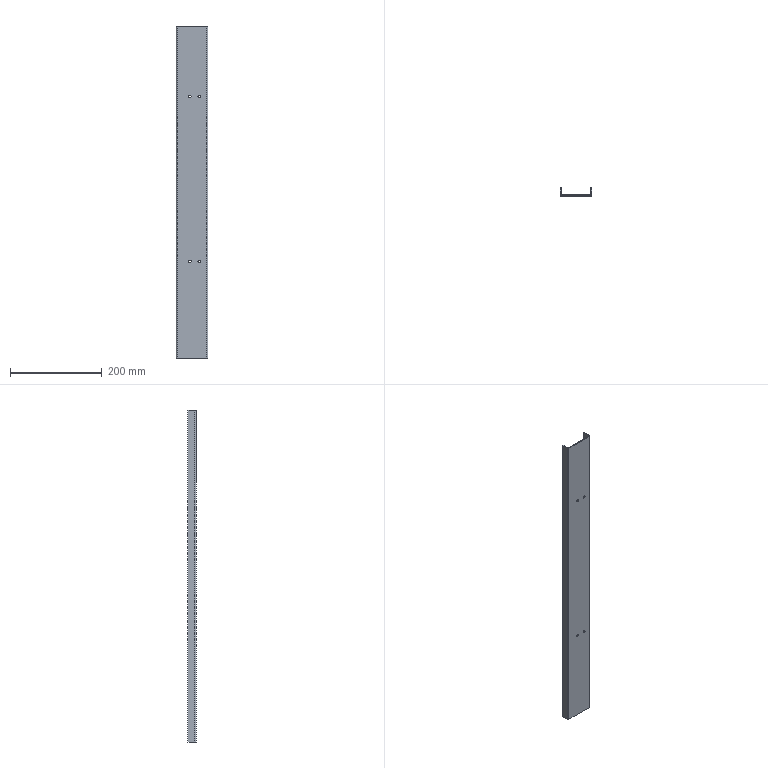Part | STEP file | PN_0020 tank-chain support plate | 1 solid | 30 faces | box 69 x 18 x 725 mm | volume 144131 mm3 | plane 18 | cylinder 12 | commonest cylinder face diameters 5 x8 1.473 x2 5.473 x2